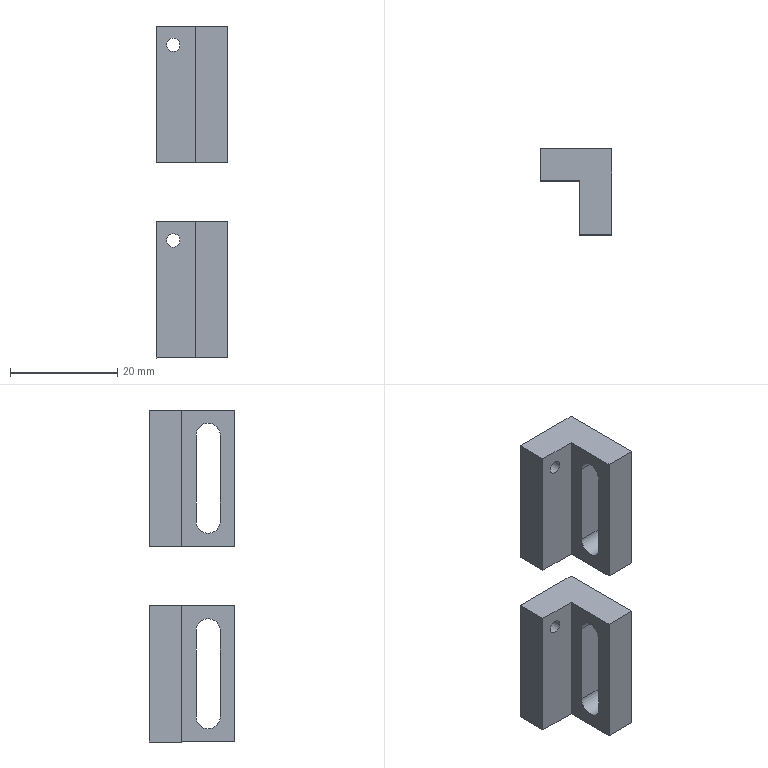CAM job | NX | 3+2 milling | part box 13.4 x 16 x 61.8 mm | stock box 20 x 21 x 66.8 mm
Tools:
number,name,description,diameter,corner_radius,flute_length,length,flutes
4,D4,平底铣刀-粗,4.0,0.0,25.0,75.0,2
9,D10,平底铣刀-粗,10.0,0.0,35.0,75.0,2
11,D4-J,平底铣刀-精,4.0,0.0,50.0,75.0,2
10,D10-J,平底铣刀-精,10.0,0.0,35.0,75.0,2
1,D80R0.8飞刀,圆鼻刀-粗,80.0,0.8,50.0,75.0,2
2,D6倒角刀,倒角刀,6.0,0.0,3.0,25.0,2
Operations:
program,operation,operation_type,tool,method,geometry_group,spindle_rpm,surface_speed,feed_per_tooth,feed_cut,feed_plunge,cut_length_mm,path_length_mm,cut_time_min,machine_time_min
A,顶面,FaceMilling,D80R0.8飞刀,侧刃精光-切深K-步距G,W-A,4000.0,1005.31,0.125,1000.0,100.0,155.8,191.8,0.1558,0.1594
A,外形粗_2,VolumeBased25DMillingOperation,D10,METHOD,W-A,8000.0,251.327,0.3125,5000.0,80.0,4367.182,4507.882,0.8734,0.8875
A,底壁粗_1,VolumeBased25DMillingOperation,D10,METHOD,W-A,8000.0,251.327,0.2188,3500.0,100.0,2253.0,2621.511,0.6437,0.6806
A,通腰槽粗_1,VolumeBased25DMillingOperation,D4,METHOD,W-A,6000.0,75.398,0.125,1500.0,100.0,2440.785,2596.285,1.627,1.643
A,腰槽精_1,VolumeBased25DMillingOperation,D4-J,METHOD,W-A,6000.0,113.0,0.0417,500.0,100.0,143.196,329.096,0.2864,0.305
A,仅选体,SurfaceContour,D6倒角刀,METHOD,W-A,8000.0,150.796,0.1875,3000.0,100.0,407.291,738.217,0.1358,0.1689
A,底精_1,VolumeBased25DMillingOperation,D10-J,METHOD,W-A,6000.0,113.0,0.2083,1200.0,100.0,173.3,318.04,0.1444,0.1589
A,底侧精_3,VolumeBased25DMillingOperation,D10-J,METHOD,W-A,6000.0,113.0,0.2083,1200.0,100.0,77.483,257.863,0.0646,0.0826
A,外形半精_2,VolumeBased25DMillingOperation,D10-J,METHOD,W-A,8000.0,251.327,0.0625,1000.0,100.0,238.432,418.632,0.2384,0.2565